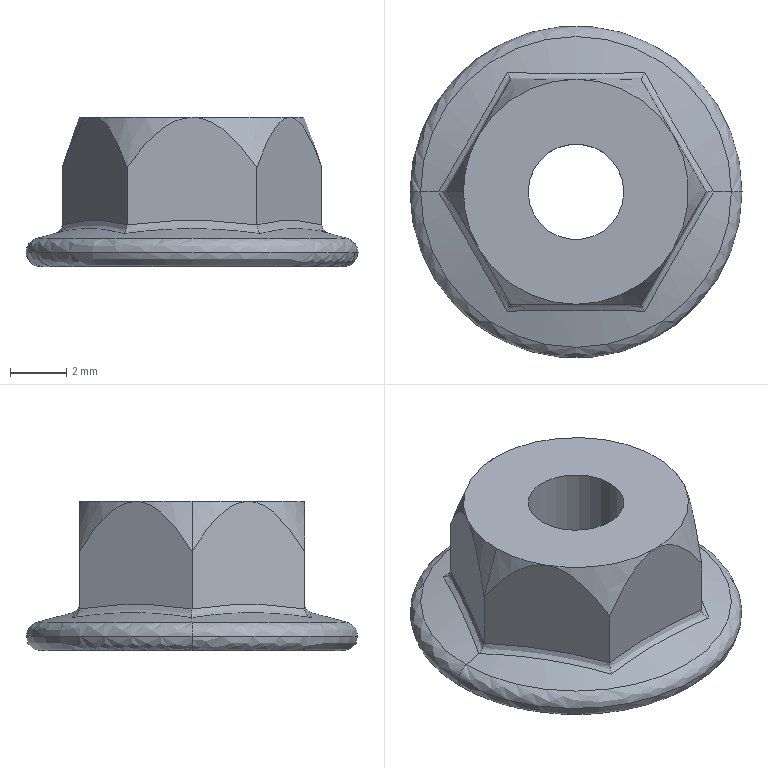Part | STEP file | prevailing torque hex nuts with flange gb_PreviewCfg | 1 solid | 31 faces | box 11.8 x 11.8 x 5.3 mm | volume 298.912 mm3 | cone 11 | spline 10 | plane 8 | cylinder 2 | commonest cylinder face diameters 3.4 x2